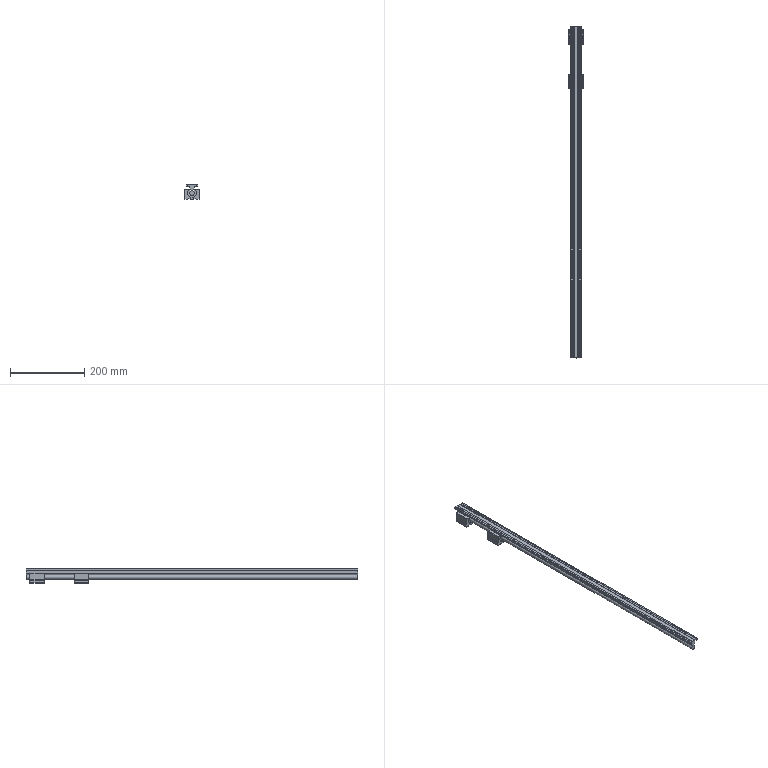Part | SolidWorks | 3 solids | 231 faces | box 40 x 895 x 39.5 mm | volume 383504 mm3 | plane 147 | cylinder 68 | cone 16 | commonest cylinder face diameters 4.5 x32 4.2 x20 12 x6 24 x6 5 x4